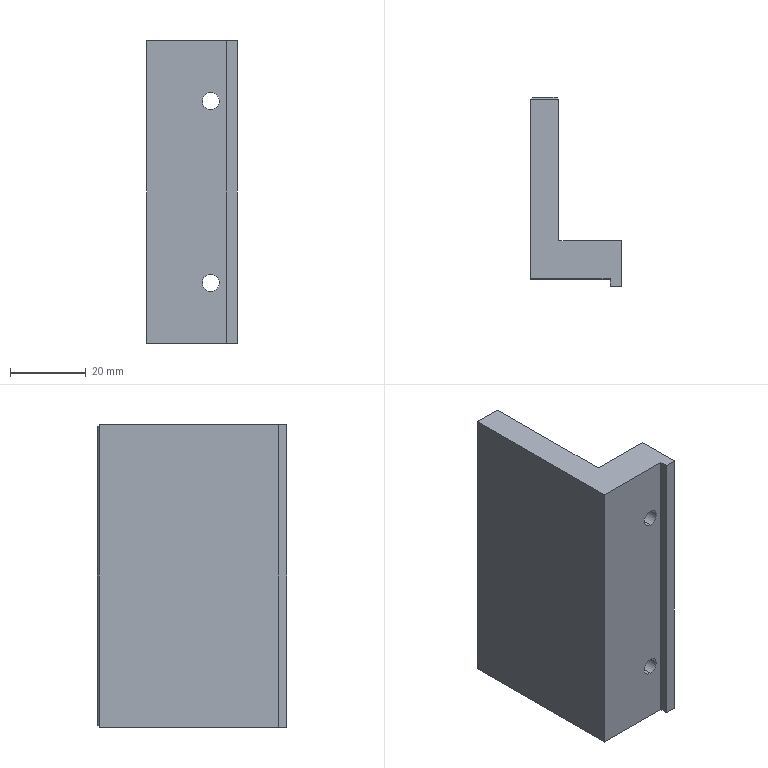Part | STEP file | 2066 Adapter plate | 1 solid | 24 faces | box 24 x 50 x 80 mm | volume 41824 mm3 | plane 16 | cylinder 8 | commonest cylinder face diameters 4.5 x4 8 x4